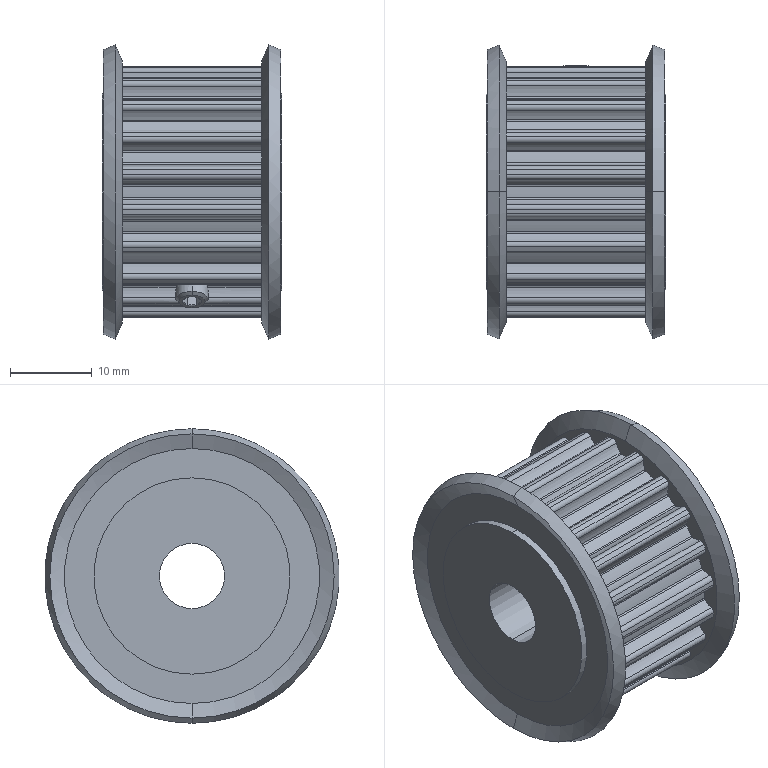Part | STEP file | HTPA20S5M150-A-P9 | 2 solids | 262 faces | box 22 x 36 x 36 mm | volume 14035 mm3 | cylinder 204 | cone 34 | plane 24 | commonest cylinder face diameters 1.1 x53 0.5 x45 6.55 x44 27.33 x22 30.87 x21 3.242 x6